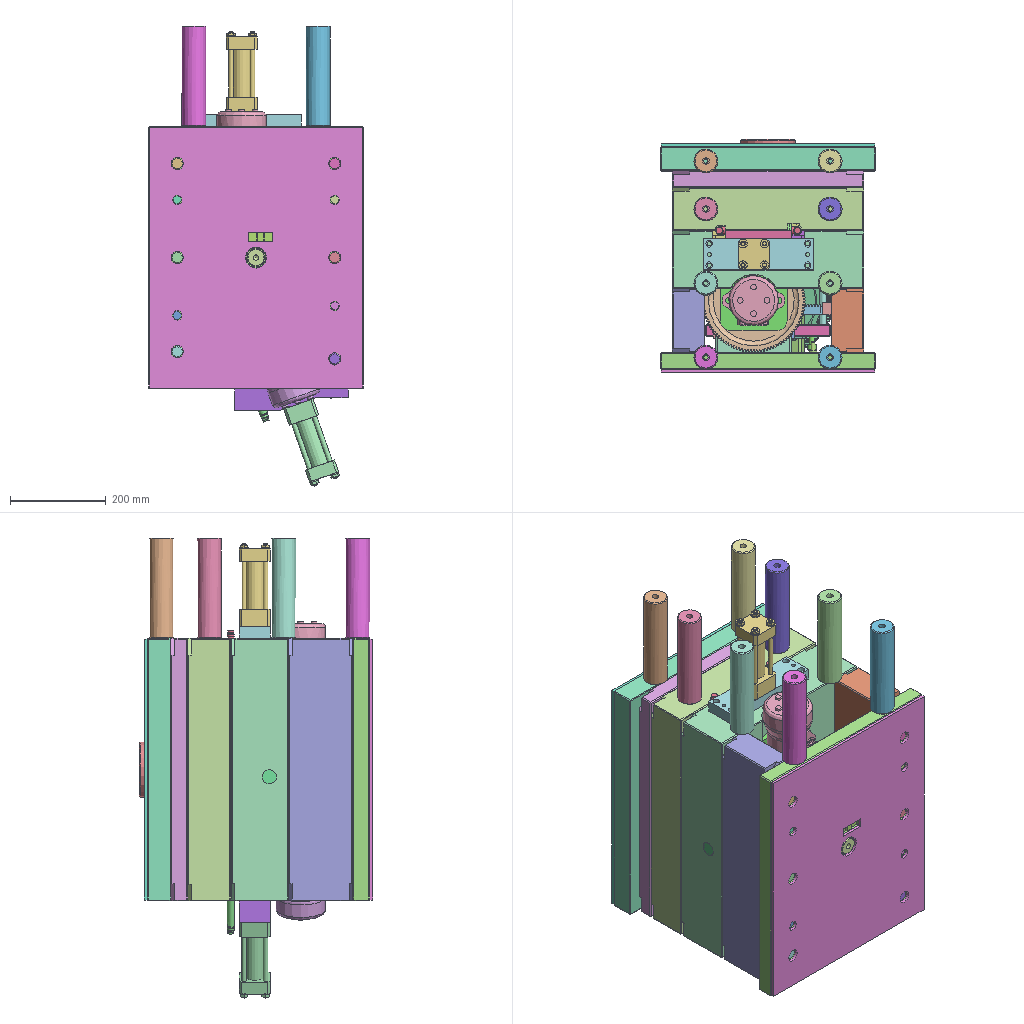Assembly | STEP file | 175 different items | 175 placed | box 450 x 488 x 963 mm
Parts list (item | name | quantity | size | volume):
1 | A-PLATE_id546_x_t | x1 | 400 x 90 x 550 mm | 14561004 mm3
2 | B-PLATE-INSERT_id78_x_t | x1 | 32 x 10 x 56 mm | 14165 mm3
3 | B-PLATE-INSERT_id82_x_t | x1 | 56 x 10 x 32 mm | 14165 mm3
4 | B-PLATE-INSERT_id86_x_t | x1 | 32 x 10 x 56 mm | 14165 mm3
5 | B-PLATE-INSERT_id90_x_t | x1 | 56 x 10 x 32 mm | 13802 mm3
6 | B-PLATE_id558_x_t | x1 | 400 x 120 x 550 mm | 16282853 mm3
7 | BOTTOM-CLAMP-PLATE_id494_x_t | x1 | 450 x 35 x 550 mm | 8473863 mm3
8 | BRONZE-BUSH1_id526_x_t | x1 | 69.598 x 71 x 31.241 mm | 9054 mm3
9 | BRONZE-BUSH1_id530_x_t | x1 | 69.598 x 71 x 31.241 mm | 9054 mm3
10 | BRONZE-BUSH2_id534_x_t | x1 | 71 x 71 x 8 mm | 9802 mm3
11 | BRONZE-BUSH2_id538_x_t | x1 | 71 x 71 x 8 mm | 9802 mm3
12 | CAV_id650_x_t | x1 | 200 x 60 x 95 mm | 908524 mm3
13 | COOLING-CAV_id202_x_t | x1 | 267.068 x 59.568 x 76.003 mm | 57701 mm3
14 | COOLING-COR_id198_x_t | x1 | 400 x 64.384 x 90 mm | 53366 mm3
15 | COOLING-SLIDE1_id166_x_t | x1 | 203.633 x 17.057 x 244.616 mm | 86128 mm3
16 | COOLING-SLIDE2_id162_x_t | x1 | 180 x 16.813 x 255.984 mm | 79230 mm3
17 | COR_id646_x_t | x1 | 200 x 60 x 90 mm | 873749 mm3
18 | EJECTION-COUPLING-SHANK_id458_x_t | x1 | 44 x 75 x 52 mm | 81524 mm3
19 | EJECTION-PIN_id142_x_t | x1 | 10 x 198.09 x 8.5 mm | 4042 mm3
20 | EJECTION-PIN_id146_x_t | x1 | 10 x 200.49 x 8.5 mm | 4074 mm3
21 | EJECTION-PIN_id150_x_t | x1 | 10 x 194.406 x 8.5 mm | 3970 mm3
22 | EJECTION-PLATE_id490_x_t | x1 | - | -
23 | EJECTION-REMAINER-PLATE_id486_x_t | x1 | 260 x 25 x 105 mm | 607320 mm3
24 | ELECTRICAL-MICRO-SWITCH1_id38_x_t | x1 | 52 x 18 x 50 mm | 21085 mm3
25 | ELECTRICAL-MICRO-SWITCH1_id42_x_t | x1 | 12.5 x 3.8 x 12.5 mm | 464.776 mm3
26 | ELECTRICAL-MICRO-SWITCH1_id46_x_t | x1 | 12.5 x 3.8 x 12.5 mm | 464.776 mm3
27 | ELECTRICAL-MICRO-SWITCH1_id50_x_t | x1 | 51.939 x 18 x 53.975 mm | 21085 mm3
28 | ELECTRICAL-MICRO-SWITCH1_id54_x_t | x1 | 12.5 x 3.8 x 12.5 mm | 464.776 mm3
29 | ELECTRICAL-MICRO-SWITCH1_id58_x_t | x1 | 12.5 x 3.8 x 12.5 mm | 464.776 mm3
30 | ELECTRICAL-MICRO-SWITCH1_id62_x_t | x1 | 52 x 18 x 50 mm | 21085 mm3
31 | ELECTRICAL-MICRO-SWITCH1_id66_x_t | x1 | 51.939 x 18 x 53.975 mm | 21085 mm3
32 | ELECTRICAL-MICRO-SWITCH2_id22_x_t | x1 | 50 x 52 x 18 mm | 21085 mm3
33 | ELECTRICAL-MICRO-SWITCH2_id26_x_t | x1 | 50 x 52 x 18 mm | 21085 mm3
34 | ELECTRICAL-MICRO-SWITCH2_id30_x_t | x1 | 12.5 x 12.5 x 3.8 mm | 464.776 mm3
35 | ELECTRICAL-MICRO-SWITCH2_id34_x_t | x1 | 12.5 x 12.5 x 3.8 mm | 464.776 mm3
36 | ELECTRICAL-MICRO-SWITCH3_id10_x_t | x1 | 53.141 x 52 x 33.658 mm | 21085 mm3
37 | ELECTRICAL-MICRO-SWITCH3_id14_x_t | x1 | 53.141 x 52 x 33.658 mm | 21085 mm3
38 | ELECTRICAL-MICRO-SWITCH3_id18_x_t | x1 | 12.918 x 12.5 x 7.621 mm | 464.776 mm3
39 | ELECTRICAL-MICRO-SWITCH3_id6_x_t | x1 | 12.918 x 12.5 x 7.621 mm | 464.776 mm3
40 | ELECTRICAL-MICRO-SWITCH4_id694_x_t | x1 | 50 x 52 x 18 mm | 21085 mm3
41 | ELECTRICAL-MICRO-SWITCH4_id698_x_t | x1 | 12.5 x 12.5 x 3.8 mm | 464.776 mm3
42 | GEAR1-1_id514_x_t | x1 | 87.142 x 83.945 x 56.458 mm | 75327 mm3
43 | GEAR1-2_id418_x_t | x1 | 226.977 x 215.948 x 138.087 mm | 1339603 mm3
44 | GEAR1-3_id414_x_t | x1 | 32.638 x 23.177 x 46.405 mm | 10951 mm3
45 | GEAR2-1_id518_x_t | x1 | 83.945 x 83.945 x 39 mm | 75327 mm3
46 | GEAR2-2_id446_x_t | x1 | 216 x 215.948 x 42.5 mm | 942512 mm3
47 | GEAR2-3_id442_x_t | x1 | 24 x 23.177 x 42.5 mm | 10951 mm3
48 | GUIDE-PIN_id286_x_t | x1 | 40 x 349.996 x 40 mm | 334779 mm3
49 | GUIDE-PIN_id290_x_t | x1 | 40 x 349.996 x 40 mm | 334779 mm3
50 | GUIDE-PIN_id294_x_t | x1 | 40 x 349.996 x 40 mm | 334779 mm3
51 | GUIDE-PIN_id298_x_t | x1 | 40 x 349.996 x 40 mm | 334779 mm3
52 | GUIDE1_id270_x_t | x1 | 47 x 35 x 47 mm | 26873 mm3
53 | GUIDE1_id274_x_t | x1 | 47 x 35 x 47 mm | 26873 mm3
54 | GUIDE1_id278_x_t | x1 | 47 x 35 x 47 mm | 26873 mm3
55 | GUIDE1_id282_x_t | x1 | 47 x 35 x 47 mm | 26873 mm3
56 | GUIDE2_id254_x_t | x1 | 52 x 90 x 52 mm | 73227 mm3
57 | GUIDE2_id258_x_t | x1 | 52 x 90 x 52 mm | 73227 mm3
58 | GUIDE2_id262_x_t | x1 | 52 x 90 x 52 mm | 73227 mm3
59 | GUIDE2_id266_x_t | x1 | 52 x 90 x 52 mm | 73227 mm3
60 | GUIDE3_id238_x_t | x1 | 52 x 120 x 52 mm | 96373 mm3
61 | GUIDE3_id242_x_t | x1 | 52 x 120 x 52 mm | 96373 mm3
62 | GUIDE3_id246_x_t | x1 | 52 x 120 x 52 mm | 96373 mm3
63 | GUIDE3_id250_x_t | x1 | 52 x 120 x 52 mm | 96373 mm3
64 | GUIDE4_id102_x_t | x1 | 30 x 40 x 30 mm | 12807 mm3
65 | GUIDE4_id106_x_t | x1 | 30 x 40 x 30 mm | 12807 mm3
66 | GUIDE4_id94_x_t | x1 | 30 x 40 x 30 mm | 12807 mm3
67 | GUIDE4_id98_x_t | x1 | 30 x 40 x 30 mm | 12807 mm3
68 | HYDRAULIC-CYLINDER-1_id470_x_t | x1 | 127.502 x 65 x 277.497 mm | 457053 mm3
69 | HYDRAULIC-CYLINDER-2_id478_x_t | x1 | 65 x 65 x 255.997 mm | 449957 mm3
70 | HYDRAULIC-CYLINDER-BASE1_id474_x_t | x1 | 238 x 65 x 45 mm | 410025 mm3
71 | HYDRAULIC-CYLINDER-BASE2_id482_x_t | x1 | 230 x 65 x 25 mm | 350259 mm3
72 | INSULT-PLATE_id450_x_t | x1 | 446 x 6 x 546 mm | 1293142 mm3
73 | INSULT-PLATE_id454_x_t | x1 | 446 x 6 x 546 mm | 1419506 mm3
74 | LOCATING-RING_id466_x_t | x1 | 168.974 x 31 x 168.974 mm | 442112 mm3
75 | MOLD-FOOT_id206_x_t | x1 | 50 x 50 x 210 mm | 388518 mm3
76 | MOLD-FOOT_id210_x_t | x1 | 50 x 50 x 210 mm | 388518 mm3
77 | MOLD-FOOT_id214_x_t | x1 | 50 x 50 x 210 mm | 388518 mm3
78 | MOLD-FOOT_id218_x_t | x1 | 50 x 50 x 210 mm | 388518 mm3
79 | MOLD-FOOT_id222_x_t | x1 | 50 x 50 x 210 mm | 388518 mm3
80 | MOLD-FOOT_id226_x_t | x1 | 50 x 50 x 210 mm | 388518 mm3
81 | MOLD-FOOT_id230_x_t | x1 | 50 x 50 x 210 mm | 388518 mm3
82 | MOLD-FOOT_id234_x_t | x1 | 50 x 50 x 210 mm | 388518 mm3
83 | MOTOR-BASE1_id426_x_t | x1 | 155.335 x 125 x 111.336 mm | 504063 mm3
84 | MOTOR-BASE2_id438_x_t | x1 | 140 x 125 x 70 mm | 504063 mm3
85 | MOTOR1_id422_x_t | x1 | - | 1091515 mm3
86 | MOTOR2_id434_x_t | x1 | 130 x 105 x 207.5 mm | 1082578 mm3
87 | RACK-BASE1_id406_x_t | x1 | 176.925 x 89.028 x 85.6 mm | 452373 mm3
88 | RACK-BASE2_id654_x_t | x1 | 160 x 89.028 x 30 mm | 401916 mm3
89 | RACK1-INSERT_id678_x_t | x1 | 23.86 x 15 x 20.816 mm | 4125 mm3
90 | RACK1_id410_x_t | x1 | 186.352 x 20.596 x 72.41 mm | 67641 mm3
91 | RACK2-INSERT_id682_x_t | x1 | 20 x 15 x 15 mm | 4125 mm3
92 | RACK2_id430_x_t | x1 | 160 x 20.596 x 30 mm | 72119 mm3
93 | RETURN-PIN_id302_x_t | x1 | 21 x 221 x 21 mm | 44798 mm3
94 | RETURN-PIN_id306_x_t | x1 | 21 x 221 x 21 mm | 44798 mm3
95 | RETURN-PIN_id310_x_t | x1 | 21 x 221 x 21 mm | 44798 mm3
96 | RETURN-PIN_id314_x_t | x1 | 21 x 221 x 21 mm | 44798 mm3
97 | RUNNER-PIN_id154_x_t | x1 | 12 x 60.5 x 12 mm | 2342 mm3
98 | RUNNER_id158_x_t | x1 | 76.069 x 81.16 x 32.686 mm | 5385 mm3
99 | SCREW-1_id382_x_t | x1 | 24 x 209.351 x 24 mm | 45976 mm3
100 | SCREW-1_id386_x_t | x1 | 24 x 209.351 x 24 mm | 45976 mm3
101 | SCREW-1_id390_x_t | x1 | 24 x 209.351 x 24 mm | 45976 mm3
102 | SCREW-1_id394_x_t | x1 | 24 x 209.351 x 24 mm | 45976 mm3
103 | SCREW-1_id398_x_t | x1 | 24 x 209.351 x 24 mm | 45976 mm3
104 | SCREW-1_id402_x_t | x1 | 24 x 209.351 x 24 mm | 45976 mm3
105 | SCREW-2_id366_x_t | x1 | 18 x 55 x 18 mm | 7891 mm3
106 | SCREW-2_id370_x_t | x1 | 18 x 55 x 18 mm | 7891 mm3
107 | SCREW-2_id374_x_t | x1 | 18 x 55 x 18 mm | 7891 mm3
108 | SCREW-2_id378_x_t | x1 | 18 x 55 x 18 mm | 7891 mm3
109 | SCREW-3_id350_x_t | x1 | 18.939 x 46.759 x 18.939 mm | 6355 mm3
110 | SCREW-3_id354_x_t | x1 | 18.939 x 46.759 x 18.939 mm | 6355 mm3
111 | SCREW-3_id358_x_t | x1 | 18.939 x 46.759 x 18.939 mm | 6355 mm3
112 | SCREW-3_id362_x_t | x1 | 18.939 x 46.759 x 18.939 mm | 6355 mm3
113 | SCREW-4_id658_x_t | x1 | 30 x 71 x 30 mm | 25054 mm3
114 | SCREW-4_id662_x_t | x1 | 30 x 71 x 30 mm | 25054 mm3
115 | SCREW-4_id666_x_t | x1 | 30 x 71 x 30 mm | 25054 mm3
116 | SCREW-4_id670_x_t | x1 | 30 x 71 x 30 mm | 25054 mm3
117 | SCREW-5_id334_x_t | x1 | 30 x 231 x 30 mm | 75324 mm3
118 | SCREW-5_id338_x_t | x1 | 30 x 231 x 30 mm | 75324 mm3
119 | SCREW-5_id342_x_t | x1 | 30 x 231 x 30 mm | 75324 mm3
120 | SCREW-5_id346_x_t | x1 | 30 x 231 x 30 mm | 75324 mm3
121 | SCREW-BUSH1_id522_x_t | x1 | 80.202 x 74 x 44.89 mm | 42151 mm3
122 | SCREW-BUSH2_id542_x_t | x1 | 80 x 75 x 22.5 mm | 49484 mm3
123 | SLIDE1-1_id622_x_t | x1 | 154.532 x 120 x 85.769 mm | 429679 mm3
124 | SLIDE1-2_id582_x_t | x1 | 161.375 x 120 x 111.146 mm | 535802 mm3
125 | SLIDE1-3_id578_x_t | x1 | - | -
126 | SLIDE1-INSERT1_id642_x_t | x1 | 129.599 x 68 x 243.479 mm | 360421 mm3
127 | SLIDE1-INSERT2_id638_x_t | x1 | 38.941 x 23.516 x 61.041 mm | 21493 mm3
128 | SLIDE1-INSERT3_id690_x_t | x1 | 20.917 x 13.3 x 35.438 mm | 1710 mm3
129 | SLIDE1-INSERT_id74_x_t | x1 | 19.863 x 14 x 22.445 mm | 3561 mm3
130 | SLIDE1-LIFTER1_id634_x_t | x1 | 43.318 x 14 x 75.744 mm | 9406 mm3
131 | SLIDE1-LIFTER2_id630_x_t | x1 | 43.318 x 14 x 75.744 mm | 9406 mm3
132 | SLIDE1-PLATE_id550_x_t | x1 | 110.798 x 59.5 x 232 mm | 275836 mm3
133 | SLIDE1-PLATE_id554_x_t | x1 | 100.862 x 59.5 x 216.856 mm | 259316 mm3
134 | SLIDE1-SCEW-AXS_id626_x_t | x1 | 101.763 x 59.001 x 162.348 mm | 124425 mm3
135 | SLIDE2-1_id618_x_t | x1 | - | -
136 | SLIDE2-2_id594_x_t | x1 | 168 x 120 x 43 mm | 457248 mm3
137 | SLIDE2-3_id590_x_t | x1 | 168 x 120 x 45 mm | 525996 mm3
138 | SLIDE2-4_id586_x_t | x1 | - | -
139 | SLIDE2-INSERT1_id614_x_t | x1 | 59 x 61 x 201.385 mm | 145141 mm3
140 | SLIDE2-INSERT2_id610_x_t | x1 | 34 x 32.5 x 57.321 mm | 25904 mm3
141 | SLIDE2-INSERT_id70_x_t | x1 | 15.757 x 14 x 20 mm | 3560 mm3
142 | SLIDE2-LIFTER1_id606_x_t | x1 | 10 x 12 x 42 mm | 2766 mm3
143 | SLIDE2-PLATE_id562_x_t | x1 | 27 x 59.5 x 213.003 mm | 241757 mm3
144 | SLIDE2-PLATE_id566_x_t | x1 | 27 x 59.5 x 213.003 mm | 241757 mm3
145 | SLIDE2-SCREW-AXS_id598_x_t | x1 | 60.006 x 59.998 x 132.392 mm | 194092 mm3
146 | SLIDE2LIFTER2_id602_x_t | x1 | 10 x 12 x 42 mm | 2766 mm3
147 | SPACE-OLATE-INSERT_id702_x_t | x1 | 17.329 x 25 x 30 mm | 11989 mm3
148 | SPACE-PLATE_id498_x_t | x1 | 68 x 135 x 550 mm | 4420744 mm3
149 | SPACE-PLATE_id502_x_t | x1 | 68 x 135 x 550 mm | 4551876 mm3
150 | SPRING_id686_x_t | x1 | 22.825 x 11.499 x 37.765 mm | 1937 mm3
151 | SPRUE_id462_x_t | x1 | 100 x 70 x 100 mm | 170232 mm3
152 | STOP-PIN_id318_x_t | x1 | 16 x 23.859 x 16 mm | 1914 mm3
153 | STOP-PIN_id322_x_t | x1 | 16 x 23.859 x 16 mm | 1914 mm3
154 | STOP-PIN_id326_x_t | x1 | 16 x 23.859 x 16 mm | 1914 mm3
155 | STOP-PIN_id330_x_t | x1 | 16 x 23.859 x 16 mm | 1914 mm3
156 | SUPPORT-PLATE_id510_x_t | x1 | 400 x 35 x 550 mm | 7237990 mm3
157 | T-BLOCK1_id174_x_t | x1 | 32.854 x 26 x 32.245 mm | 15406 mm3
158 | T-BLOCK2_id178_x_t | x1 | 32 x 29.5 x 25 mm | 17357 mm3
159 | TOP-CLAMP-PLATE_id506_x_t | x1 | 450 x 50 x 550 mm | 11584870 mm3
160 | WEAR-PLATE1_id182_x_t | x1 | 140 x 6 x 77 mm | 64551 mm3
161 | WEAR-PLATE1_id186_x_t | x1 | 140 x 6 x 32 mm | 26706 mm3
162 | WEAR-PLATE1_id190_x_t | x1 | 122.87 x 6 x 72.641 mm | 26871 mm3
163 | WEAR-PLATE1_id194_x_t | x1 | 127.71 x 6 x 86.31 mm | 37311 mm3
164 | WEAR-PLATE2_id674_x_t | x1 | 140 x 83.443 x 25.901 mm | 68382 mm3
165 | WEAR-PLATE3_id170_x_t | x1 | 118.359 x 83.443 x 62.371 mm | 58708 mm3
166 | WEDGE-1_id570_x_t | x1 | 128.423 x 82.5 x 83.604 mm | 350596 mm3
167 | WEDGE-2_id574_x_t | x1 | 138 x 82.5 x 48.5 mm | 384224 mm3
168 | Z05-16-1_id126_x_t | x1 | 15.681 x 23 x 15.681 mm | 3250 mm3
169 | Z05-16-1_id130_x_t | x1 | 15.681 x 23 x 15.681 mm | 3250 mm3
170 | Z05-16-1_id134_x_t | x1 | 15.681 x 23 x 15.681 mm | 3250 mm3
171 | Z05-16-1_id138_x_t | x1 | 15.681 x 23 x 15.681 mm | 3250 mm3
172 | Z05-16-2_id110_x_t | x1 | 15.681 x 16 x 15.681 mm | 2631 mm3
173 | Z05-16-2_id114_x_t | x1 | 15.681 x 16 x 15.681 mm | 2631 mm3
174 | Z05-16-2_id118_x_t | x1 | 15.681 x 16 x 15.681 mm | 2631 mm3
175 | Z05-16-2_id122_x_t | x1 | 15.681 x 16 x 15.681 mm | 2631 mm3